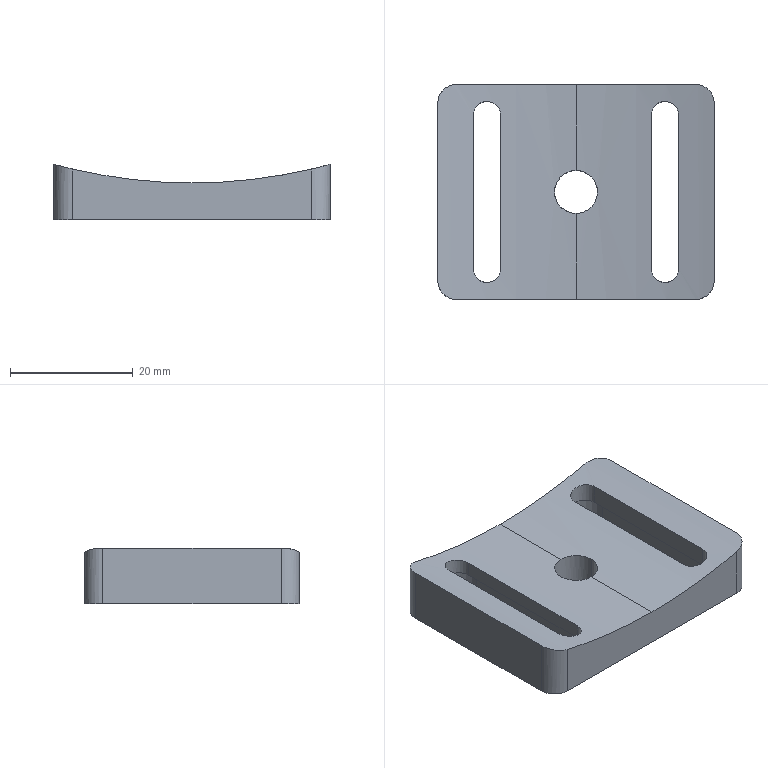Part | SolidWorks | features ICE 2, Extrusion 1, Fillet 1, HoleWzd 1 | 1 solid | 31 faces | box 45 x 35 x 9.032 mm | volume 7770 mm3 | cylinder 16 | plane 15 | commonest cylinder face diameters 4.5 x4 6 x4 8 x4 7 x2 170 x2
STEP:
#1=CARTESIAN_POINT('',(3.5,17.5,-84.928));
#2=VERTEX_POINT('',#1);
#3=CARTESIAN_POINT('',(0.,14.,-85.));
#4=VERTEX_POINT('',#3);
#5=CARTESIAN_POINT('',(3.5,17.5,-84.928));
#6=CARTESIAN_POINT('',(3.5,17.271,-84.928));
#7=CARTESIAN_POINT('',(3.478,17.044,-84.929));
#8=CARTESIAN_POINT('',(3.388,16.593,-84.932));
#9=CARTESIAN_POINT('',(3.321,16.372,-84.935));
#10=CARTESIAN_POINT('',(3.146,15.95,-84.942));
#11=CARTESIAN_POINT('',(3.038,15.747,-84.946));
#12=CARTESIAN_POINT('',(2.782,15.364,-84.955));
#13=CARTESIAN_POINT('',(2.637,15.187,-84.959));
#14=CARTESIAN_POINT('',(2.314,14.864,-84.969));
#15=CARTESIAN_POINT('',(2.134,14.717,-84.973));
#16=CARTESIAN_POINT('',(1.753,14.462,-84.982));
#17=CARTESIAN_POINT('',(1.552,14.355,-84.986));
#18=CARTESIAN_POINT('',(1.129,14.179,-84.993));
#19=CARTESIAN_POINT('',(0.906,14.112,-84.995));
#20=CARTESIAN_POINT('',(0.4583,14.023,-84.999));
#21=CARTESIAN_POINT('',(0.231,14.,-85.));
#22=CARTESIAN_POINT('',(0.,14.,-85.));
#23=B_SPLINE_CURVE_WITH_KNOTS('',3,(#5,#6,#7,#8,#9,#10,#11,#12,#13,#14,#15,#16,#17,#18,#19,#20,#21,#22),.UNSPECIFIED.,.F.,.F.,(4,2,2,2,2,2,2,2,4),(0.01094,0.01163,0.01231,0.013,0.01368,0.01436,0.01505,0.01573,0.01642),.UNSPECIFIED.);
#24=EDGE_CURVE('',#2,#4,#23,.T.);
#25=ORIENTED_EDGE('',*,*,#24,.F.);
#26=CARTESIAN_POINT('',(3.5,17.5,-91.));
#27=VERTEX_POINT('',#26);
#28=CARTESIAN_POINT('',(3.5,17.5,-91.));
#29=DIRECTION('',(0.,0.,-1.));
#30=VECTOR('',#29,1000.);
#31=LINE('',#28,#30);
#32=EDGE_CURVE('',#2,#27,#31,.T.);
#33=ORIENTED_EDGE('',*,*,#32,.T.);
#34=CARTESIAN_POINT('',(-3.5,17.5,-91.));
#35=VERTEX_POINT('',#34);
#36=CARTESIAN_POINT('',(0.,17.5,-91.));
#37=DIRECTION('',(0.,0.,-1.));
#38=DIRECTION('',(-1.,0.,0.));
#39=AXIS2_PLACEMENT_3D('',#36,#37,#38);
#40=CIRCLE('',#39,3.5);
#41=EDGE_CURVE('',#27,#35,#40,.T.);
#42=ORIENTED_EDGE('',*,*,#41,.T.);
#43=CARTESIAN_POINT('',(-3.5,17.5,-84.928));
#44=VERTEX_POINT('',#43);
#45=CARTESIAN_POINT('',(-3.5,17.5,-91.));
#46=DIRECTION('',(0.,0.,-1.));
#47=VECTOR('',#46,1000.);
#48=LINE('',#45,#47);
#49=EDGE_CURVE('',#44,#35,#48,.T.);
#50=ORIENTED_EDGE('',*,*,#49,.F.);
#51=CARTESIAN_POINT('',(0.,14.,-85.));
#52=CARTESIAN_POINT('',(-0.2307,14.,-85.));
#53=CARTESIAN_POINT('',(-0.4588,14.023,-84.999));
#54=CARTESIAN_POINT('',(-0.9058,14.112,-84.995));
#55=CARTESIAN_POINT('',(-1.128,14.179,-84.993));
#56=CARTESIAN_POINT('',(-1.552,14.354,-84.986));
#57=CARTESIAN_POINT('',(-1.753,14.462,-84.982));
#58=CARTESIAN_POINT('',(-2.133,14.715,-84.973));
#59=CARTESIAN_POINT('',(-2.313,14.863,-84.969));
#60=CARTESIAN_POINT('',(-2.636,15.186,-84.959));
#61=CARTESIAN_POINT('',(-2.78,15.362,-84.955));
#62=CARTESIAN_POINT('',(-3.036,15.743,-84.946));
#63=CARTESIAN_POINT('',(-3.145,15.947,-84.942));
#64=CARTESIAN_POINT('',(-3.407,16.579,-84.932));
#65=CARTESIAN_POINT('',(-3.5,17.038,-84.928));
#66=CARTESIAN_POINT('',(-3.5,17.5,-84.928));
#67=B_SPLINE_CURVE_WITH_KNOTS('',3,(#51,#52,#53,#54,#55,#56,#57,#58,#59,#60,#61,#62,#63,#64,#65,#66),.UNSPECIFIED.,.F.,.F.,(4,2,2,2,2,2,2,4),(0.01642,0.0171,0.01778,0.01847,0.01915,0.01983,0.02052,0.02189),.UNSPECIFIED.);
#68=EDGE_CURVE('',#4,#44,#67,.T.);
#69=ORIENTED_EDGE('',*,*,#68,.F.);
#70=EDGE_LOOP('',(#25,#33,#42,#50,#69));
#71=FACE_OUTER_BOUND('',#70,.T.);
#72=CARTESIAN_POINT('',(0.,17.5,-91.));
#73=DIRECTION('',(0.,0.,-1.));
#74=DIRECTION('',(-1.,0.,0.));
#75=AXIS2_PLACEMENT_3D('',#72,#73,#74);
#76=CYLINDRICAL_SURFACE('',#75,3.5);
#77=ADVANCED_FACE('',(#71),#76,.F.);
#78=CARTESIAN_POINT('',(12.25,5.,-84.113));
#79=VERTEX_POINT('',#78);
#80=CARTESIAN_POINT('',(12.25,30.,-84.113));
#81=VERTEX_POINT('',#80);
#82=CARTESIAN_POINT('',(12.25,35.,-84.113));
#83=DIRECTION('',(0.,1.,0.));
#84=VECTOR('',#83,1000.);
#85=LINE('',#82,#84);
#86=EDGE_CURVE('',#79,#81,#85,.T.);
#87=ORIENTED_EDGE('',*,*,#86,.T.);
#88=CARTESIAN_POINT('',(16.75,30.,-83.333));
#89=VERTEX_POINT('',#88);
#90=CARTESIAN_POINT('',(12.25,30.,-84.113));
#91=CARTESIAN_POINT('',(12.25,30.15,-84.113));
#92=CARTESIAN_POINT('',(12.265,30.297,-84.11));
#93=CARTESIAN_POINT('',(12.323,30.587,-84.102));
#94=CARTESIAN_POINT('',(12.367,30.73,-84.096));
#95=CARTESIAN_POINT('',(12.481,31.004,-84.079));
#96=CARTESIAN_POINT('',(12.551,31.134,-84.068));
#97=CARTESIAN_POINT('',(12.716,31.379,-84.044));
#98=CARTESIAN_POINT('',(12.812,31.494,-84.029));
#99=CARTESIAN_POINT('',(13.125,31.805,-83.981));
#100=CARTESIAN_POINT('',(13.376,31.971,-83.941));
#101=CARTESIAN_POINT('',(13.782,32.137,-83.875));
#102=CARTESIAN_POINT('',(13.924,32.18,-83.852));
#103=CARTESIAN_POINT('',(14.212,32.236,-83.804));
#104=CARTESIAN_POINT('',(14.357,32.25,-83.779));
#105=CARTESIAN_POINT('',(14.648,32.25,-83.728));
#106=CARTESIAN_POINT('',(14.796,32.235,-83.702));
#107=CARTESIAN_POINT('',(15.082,32.178,-83.651));
#108=CARTESIAN_POINT('',(15.222,32.136,-83.626));
#109=CARTESIAN_POINT('',(15.492,32.025,-83.576));
#110=CARTESIAN_POINT('',(15.623,31.955,-83.552));
#111=CARTESIAN_POINT('',(15.866,31.794,-83.506));
#112=CARTESIAN_POINT('',(15.98,31.701,-83.484));
#113=CARTESIAN_POINT('',(16.19,31.493,-83.444));
#114=CARTESIAN_POINT('',(16.284,31.379,-83.426));
#115=CARTESIAN_POINT('',(16.448,31.136,-83.393));
#116=CARTESIAN_POINT('',(16.519,31.004,-83.379));
#117=CARTESIAN_POINT('',(16.633,30.73,-83.357));
#118=CARTESIAN_POINT('',(16.676,30.59,-83.348));
#119=CARTESIAN_POINT('',(16.735,30.3,-83.336));
#120=CARTESIAN_POINT('',(16.75,30.15,-83.333));
#121=CARTESIAN_POINT('',(16.75,30.,-83.333));
#122=B_SPLINE_CURVE_WITH_KNOTS('',3,(#90,#91,#92,#93,#94,#95,#96,#97,#98,#99,#100,#101,#102,#103,#104,#105,#106,#107,#108,#109,#110,#111,#112,#113,#114,#115,#116,#117,#118,#119,#120,#121),.UNSPECIFIED.,.F.,.F.,(4,2,2,2,2,2,2,2,2,2,2,2,2,2,2,4),(0.,0.0004429,0.0008859,0.001329,0.001772,0.002658,0.003101,0.003543,0.003986,0.004429,0.004872,0.005315,0.005758,0.006201,0.006644,0.007087),.UNSPECIFIED.);
#123=EDGE_CURVE('',#81,#89,#122,.T.);
#124=ORIENTED_EDGE('',*,*,#123,.T.);
#125=CARTESIAN_POINT('',(16.75,5.,-83.333));
#126=VERTEX_POINT('',#125);
#127=CARTESIAN_POINT('',(16.75,35.,-83.333));
#128=DIRECTION('',(0.,-1.,0.));
#129=VECTOR('',#128,1000.);
#130=LINE('',#127,#129);
#131=EDGE_CURVE('',#89,#126,#130,.T.);
#132=ORIENTED_EDGE('',*,*,#131,.T.);
#133=CARTESIAN_POINT('',(16.75,5.,-83.333));
#134=CARTESIAN_POINT('',(16.75,4.852,-83.333));
#135=CARTESIAN_POINT('',(16.736,4.705,-83.336));
#136=CARTESIAN_POINT('',(16.677,4.413,-83.348));
#137=CARTESIAN_POINT('',(16.633,4.27,-83.357));
#138=CARTESIAN_POINT('',(16.52,3.998,-83.379));
#139=CARTESIAN_POINT('',(16.45,3.867,-83.393));
#140=CARTESIAN_POINT('',(16.284,3.621,-83.426));
#141=CARTESIAN_POINT('',(16.191,3.508,-83.444));
#142=CARTESIAN_POINT('',(15.983,3.301,-83.484));
#143=CARTESIAN_POINT('',(15.867,3.207,-83.506));
#144=CARTESIAN_POINT('',(15.624,3.045,-83.552));
#145=CARTESIAN_POINT('',(15.495,2.977,-83.576));
#146=CARTESIAN_POINT('',(15.224,2.865,-83.626));
#147=CARTESIAN_POINT('',(15.082,2.822,-83.651));
#148=CARTESIAN_POINT('',(14.797,2.765,-83.702));
#149=CARTESIAN_POINT('',(14.652,2.75,-83.728));
#150=CARTESIAN_POINT('',(14.357,2.75,-83.779));
#151=CARTESIAN_POINT('',(14.212,2.764,-83.804));
#152=CARTESIAN_POINT('',(13.926,2.82,-83.852));
#153=CARTESIAN_POINT('',(13.784,2.862,-83.875));
#154=CARTESIAN_POINT('',(13.512,2.973,-83.919));
#155=CARTESIAN_POINT('',(13.383,3.042,-83.94));
#156=CARTESIAN_POINT('',(13.138,3.203,-83.979));
#157=CARTESIAN_POINT('',(13.021,3.298,-83.997));
#158=CARTESIAN_POINT('',(12.812,3.505,-84.029));
#159=CARTESIAN_POINT('',(12.718,3.618,-84.043));
#160=CARTESIAN_POINT('',(12.553,3.863,-84.068));
#161=CARTESIAN_POINT('',(12.481,3.995,-84.079));
#162=CARTESIAN_POINT('',(12.311,4.403,-84.104));
#163=CARTESIAN_POINT('',(12.25,4.7,-84.113));
#164=CARTESIAN_POINT('',(12.25,5.,-84.113));
#165=B_SPLINE_CURVE_WITH_KNOTS('',3,(#133,#134,#135,#136,#137,#138,#139,#140,#141,#142,#143,#144,#145,#146,#147,#148,#149,#150,#151,#152,#153,#154,#155,#156,#157,#158,#159,#160,#161,#162,#163,#164),.UNSPECIFIED.,.F.,.F.,(4,2,2,2,2,2,2,2,2,2,2,2,2,2,2,4),(0.007088,0.007531,0.007974,0.008417,0.00886,0.009303,0.009746,0.01019,0.01063,0.01107,0.01152,0.01196,0.0124,0.01285,0.01329,0.01417),.UNSPECIFIED.);
#166=EDGE_CURVE('',#126,#79,#165,.T.);
#167=ORIENTED_EDGE('',*,*,#166,.T.);
#168=EDGE_LOOP('',(#87,#124,#132,#167));
#169=FACE_BOUND('',#168,.T.);
#170=CARTESIAN_POINT('',(0.,35.,-85.));
#171=VERTEX_POINT('',#170);
#172=CARTESIAN_POINT('',(19.5,35.,-82.733));
#173=VERTEX_POINT('',#172);
#174=CARTESIAN_POINT('',(0.,35.,0.));
#175=DIRECTION('',(0.,-1.,0.));
#176=DIRECTION('',(0.,0.,1.));
#177=AXIS2_PLACEMENT_3D('',#174,#175,#176);
#178=CIRCLE('',#177,85.);
#179=EDGE_CURVE('',#171,#173,#178,.T.);
#180=ORIENTED_EDGE('',*,*,#179,.F.);
#181=CARTESIAN_POINT('',(0.,21.,-85.));
#182=VERTEX_POINT('',#181);
#183=CARTESIAN_POINT('',(0.,35.,-85.));
#184=DIRECTION('',(0.,-1.,0.));
#185=VECTOR('',#184,1000.);
#186=LINE('',#183,#185);
#187=EDGE_CURVE('',#171,#182,#186,.T.);
#188=ORIENTED_EDGE('',*,*,#187,.T.);
#189=CARTESIAN_POINT('',(0.,21.,-85.));
#190=CARTESIAN_POINT('',(0.2283,21.,-85.));
#191=CARTESIAN_POINT('',(0.4601,20.977,-84.999));
#192=CARTESIAN_POINT('',(0.9089,20.888,-84.995));
#193=CARTESIAN_POINT('',(1.127,20.822,-84.993));
#194=CARTESIAN_POINT('',(1.551,20.646,-84.986));
#195=CARTESIAN_POINT('',(1.756,20.536,-84.982));
#196=CARTESIAN_POINT('',(2.135,20.283,-84.973));
#197=CARTESIAN_POINT('',(2.311,20.138,-84.969));
#198=CARTESIAN_POINT('',(2.638,19.812,-84.959));
#199=CARTESIAN_POINT('',(2.783,19.635,-84.955));
#200=CARTESIAN_POINT('',(3.036,19.256,-84.946));
#201=CARTESIAN_POINT('',(3.146,19.051,-84.942));
#202=CARTESIAN_POINT('',(3.322,18.627,-84.935));
#203=CARTESIAN_POINT('',(3.388,18.409,-84.932));
#204=CARTESIAN_POINT('',(3.477,17.96,-84.929));
#205=CARTESIAN_POINT('',(3.5,17.728,-84.928));
#206=CARTESIAN_POINT('',(3.5,17.5,-84.928));
#207=B_SPLINE_CURVE_WITH_KNOTS('',3,(#189,#190,#191,#192,#193,#194,#195,#196,#197,#198,#199,#200,#201,#202,#203,#204,#205,#206),.UNSPECIFIED.,.F.,.F.,(4,2,2,2,2,2,2,2,4),(0.005473,0.006157,0.006841,0.007525,0.008208,0.008892,0.009576,0.01026,0.01094),.UNSPECIFIED.);
#208=EDGE_CURVE('',#182,#2,#207,.T.);
#209=ORIENTED_EDGE('',*,*,#208,.T.);
#210=ORIENTED_EDGE('',*,*,#24,.T.);
#211=CARTESIAN_POINT('',(0.,0.,-85.));
#212=VERTEX_POINT('',#211);
#213=CARTESIAN_POINT('',(0.,35.,-85.));
#214=DIRECTION('',(0.,-1.,0.));
#215=VECTOR('',#214,1000.);
#216=LINE('',#213,#215);
#217=EDGE_CURVE('',#4,#212,#216,.T.);
#218=ORIENTED_EDGE('',*,*,#217,.T.);
#219=CARTESIAN_POINT('',(19.5,0.,-82.733));
#220=VERTEX_POINT('',#219);
#221=CARTESIAN_POINT('',(0.,0.,0.));
#222=DIRECTION('',(0.,-1.,0.));
#223=DIRECTION('',(0.,0.,1.));
#224=AXIS2_PLACEMENT_3D('',#221,#222,#223);
#225=CIRCLE('',#224,85.);
#226=EDGE_CURVE('',#212,#220,#225,.T.);
#227=ORIENTED_EDGE('',*,*,#226,.T.);
#228=CARTESIAN_POINT('',(22.5,3.,-81.968));
#229=VERTEX_POINT('',#228);
#230=CARTESIAN_POINT('',(19.5,0.,-82.733));
#231=CARTESIAN_POINT('',(19.696,0.,-82.687));
#232=CARTESIAN_POINT('',(19.888,0.01899,-82.641));
#233=CARTESIAN_POINT('',(20.267,0.09331,-82.549));
#234=CARTESIAN_POINT('',(20.455,0.1494,-82.502));
#235=CARTESIAN_POINT('',(20.816,0.2968,-82.412));
#236=CARTESIAN_POINT('',(20.987,0.3871,-82.369));
#237=CARTESIAN_POINT('',(21.311,0.6007,-82.285));
#238=CARTESIAN_POINT('',(21.466,0.7256,-82.245));
#239=CARTESIAN_POINT('',(21.745,1.,-82.172));
#240=CARTESIAN_POINT('',(21.87,1.15,-82.138));
#241=CARTESIAN_POINT('',(22.092,1.476,-82.079));
#242=CARTESIAN_POINT('',(22.188,1.653,-82.053));
#243=CARTESIAN_POINT('',(22.418,2.198,-81.991));
#244=CARTESIAN_POINT('',(22.5,2.597,-81.968));
#245=CARTESIAN_POINT('',(22.5,3.,-81.968));
#246=B_SPLINE_CURVE_WITH_KNOTS('',3,(#230,#231,#232,#233,#234,#235,#236,#237,#238,#239,#240,#241,#242,#243,#244,#245),.UNSPECIFIED.,.F.,.F.,(4,2,2,2,2,2,2,4),(0.,0.000595,0.00119,0.001785,0.00238,0.002975,0.00357,0.00476),.UNSPECIFIED.);
#247=EDGE_CURVE('',#220,#229,#246,.T.);
#248=ORIENTED_EDGE('',*,*,#247,.T.);
#249=CARTESIAN_POINT('',(22.5,32.,-81.968));
#250=VERTEX_POINT('',#249);
#251=CARTESIAN_POINT('',(22.5,35.,-81.968));
#252=DIRECTION('',(0.,-1.,0.));
#253=VECTOR('',#252,1000.);
#254=LINE('',#251,#253);
#255=EDGE_CURVE('',#250,#229,#254,.T.);
#256=ORIENTED_EDGE('',*,*,#255,.F.);
#257=CARTESIAN_POINT('',(22.5,32.,-81.968));
#258=CARTESIAN_POINT('',(22.5,32.201,-81.968));
#259=CARTESIAN_POINT('',(22.48,32.399,-81.973));
#260=CARTESIAN_POINT('',(22.402,32.787,-81.995));
#261=CARTESIAN_POINT('',(22.342,32.98,-82.011));
#262=CARTESIAN_POINT('',(22.188,33.346,-82.053));
#263=CARTESIAN_POINT('',(22.095,33.519,-82.078));
#264=CARTESIAN_POINT('',(21.873,33.846,-82.138));
#265=CARTESIAN_POINT('',(21.746,33.999,-82.171));
#266=CARTESIAN_POINT('',(21.329,34.41,-82.281));
#267=CARTESIAN_POINT('',(20.995,34.629,-82.367));
#268=CARTESIAN_POINT('',(20.459,34.849,-82.501));
#269=CARTESIAN_POINT('',(20.271,34.906,-82.548));
#270=CARTESIAN_POINT('',(19.889,34.981,-82.641));
#271=CARTESIAN_POINT('',(19.696,35.,-82.687));
#272=CARTESIAN_POINT('',(19.5,35.,-82.733));
#273=B_SPLINE_CURVE_WITH_KNOTS('',3,(#257,#258,#259,#260,#261,#262,#263,#264,#265,#266,#267,#268,#269,#270,#271,#272),.UNSPECIFIED.,.F.,.F.,(4,2,2,2,2,2,2,4),(0.,0.000595,0.00119,0.001785,0.00238,0.00357,0.004165,0.00476),.UNSPECIFIED.);
#274=EDGE_CURVE('',#250,#173,#273,.T.);
#275=ORIENTED_EDGE('',*,*,#274,.T.);
#276=EDGE_LOOP('',(#180,#188,#209,#210,#218,#227,#248,#256,#275));
#277=FACE_OUTER_BOUND('',#276,.T.);
#278=CARTESIAN_POINT('',(0.,35.,0.));
#279=DIRECTION('',(0.,-1.,0.));
#280=DIRECTION('',(0.,0.,-1.));
#281=AXIS2_PLACEMENT_3D('',#278,#279,#280);
#282=CYLINDRICAL_SURFACE('',#281,85.);
#283=ADVANCED_FACE('',(#169,#277),#282,.F.);
#284=CARTESIAN_POINT('',(-12.25,30.,-86.5));
#285=VERTEX_POINT('',#284);
#286=CARTESIAN_POINT('',(-16.75,30.,-86.5));
#287=VERTEX_POINT('',#286);
#288=CARTESIAN_POINT('',(-14.5,30.,-86.5));
#289=DIRECTION('',(0.,0.,1.));
#290=DIRECTION('',(-1.,0.,0.));
#291=AXIS2_PLACEMENT_3D('',#288,#289,#290);
#292=CIRCLE('',#291,2.25);
#293=EDGE_CURVE('',#285,#287,#292,.T.);
#294=ORIENTED_EDGE('',*,*,#293,.F.);
#295=CARTESIAN_POINT('',(-12.25,30.,-84.113));
#296=VERTEX_POINT('',#295);
#297=CARTESIAN_POINT('',(-12.25,30.,-81.785));
#298=DIRECTION('',(0.,0.,-1.));
#299=VECTOR('',#298,1000.);
#300=LINE('',#297,#299);
#301=EDGE_CURVE('',#296,#285,#300,.T.);
#302=ORIENTED_EDGE('',*,*,#301,.F.);
#303=CARTESIAN_POINT('',(-16.75,30.,-83.333));
#304=VERTEX_POINT('',#303);
#305=CARTESIAN_POINT('',(-16.75,30.,-83.333));
#306=CARTESIAN_POINT('',(-16.75,30.15,-83.333));
#307=CARTESIAN_POINT('',(-16.735,30.297,-83.336));
#308=CARTESIAN_POINT('',(-16.677,30.586,-83.348));
#309=CARTESIAN_POINT('',(-16.633,30.73,-83.357));
#310=CARTESIAN_POINT('',(-16.519,31.003,-83.379));
#311=CARTESIAN_POINT('',(-16.45,31.133,-83.393));
#312=CARTESIAN_POINT('',(-16.285,31.378,-83.425));
#313=CARTESIAN_POINT('',(-16.19,31.493,-83.444));
#314=CARTESIAN_POINT('',(-15.878,31.803,-83.504));
#315=CARTESIAN_POINT('',(-15.628,31.969,-83.551));
#316=CARTESIAN_POINT('',(-15.224,32.135,-83.626));
#317=CARTESIAN_POINT('',(-15.083,32.178,-83.651));
#318=CARTESIAN_POINT('',(-14.795,32.235,-83.703));
#319=CARTESIAN_POINT('',(-14.65,32.25,-83.728));
#320=CARTESIAN_POINT('',(-14.359,32.25,-83.779));
#321=CARTESIAN_POINT('',(-14.211,32.236,-83.804));
#322=CARTESIAN_POINT('',(-13.924,32.18,-83.852));
#323=CARTESIAN_POINT('',(-13.784,32.138,-83.875));
#324=CARTESIAN_POINT('',(-13.513,32.027,-83.919));
#325=CARTESIAN_POINT('',(-13.381,31.957,-83.94));
#326=CARTESIAN_POINT('',(-13.137,31.796,-83.979));
#327=CARTESIAN_POINT('',(-13.023,31.703,-83.997));
#328=CARTESIAN_POINT('',(-12.811,31.494,-84.029));
#329=CARTESIAN_POINT('',(-12.717,31.38,-84.043));
#330=CARTESIAN_POINT('',(-12.553,31.137,-84.068));
#331=CARTESIAN_POINT('',(-12.481,31.005,-84.079));
#332=CARTESIAN_POINT('',(-12.367,30.731,-84.096));
#333=CARTESIAN_POINT('',(-12.324,30.59,-84.102));
#334=CARTESIAN_POINT('',(-12.265,30.3,-84.11));
#335=CARTESIAN_POINT('',(-12.25,30.15,-84.113));
#336=CARTESIAN_POINT('',(-12.25,30.,-84.113));
#337=B_SPLINE_CURVE_WITH_KNOTS('',3,(#305,#306,#307,#308,#309,#310,#311,#312,#313,#314,#315,#316,#317,#318,#319,#320,#321,#322,#323,#324,#325,#326,#327,#328,#329,#330,#331,#332,#333,#334,#335,#336),.UNSPECIFIED.,.F.,.F.,(4,2,2,2,2,2,2,2,2,2,2,2,2,2,2,4),(0.,0.0004429,0.0008858,0.001329,0.001772,0.002658,0.0031,0.003543,0.003986,0.004429,0.004872,0.005315,0.005758,0.006201,0.006644,0.007087),.UNSPECIFIED.);
#338=EDGE_CURVE('',#304,#296,#337,.T.);
#339=ORIENTED_EDGE('',*,*,#338,.F.);
#340=CARTESIAN_POINT('',(-16.75,30.,-81.785));
#341=DIRECTION('',(0.,0.,-1.));
#342=VECTOR('',#341,1000.);
#343=LINE('',#340,#342);
#344=EDGE_CURVE('',#304,#287,#343,.T.);
#345=ORIENTED_EDGE('',*,*,#344,.T.);
#346=EDGE_LOOP('',(#294,#302,#339,#345));
#347=FACE_OUTER_BOUND('',#346,.T.);
#348=CARTESIAN_POINT('',(-14.5,30.,-81.785));
#349=DIRECTION('',(0.,0.,-1.));
#350=DIRECTION('',(-1.,0.,0.));
#351=AXIS2_PLACEMENT_3D('',#348,#349,#350);
#352=CYLINDRICAL_SURFACE('',#351,2.25);
#353=ADVANCED_FACE('',(#347),#352,.F.);
#354=CARTESIAN_POINT('',(-16.75,5.,-86.5));
#355=VERTEX_POINT('',#354);
#356=CARTESIAN_POINT('',(-16.75,30.,-86.5));
#357=DIRECTION('',(0.,-1.,0.));
#358=VECTOR('',#357,1000.);
#359=LINE('',#356,#358);
#360=EDGE_CURVE('',#287,#355,#359,.T.);
#361=ORIENTED_EDGE('',*,*,#360,.F.);
#362=ORIENTED_EDGE('',*,*,#344,.F.);
#363=CARTESIAN_POINT('',(-16.75,5.,-83.333));
#364=VERTEX_POINT('',#363);
#365=CARTESIAN_POINT('',(-16.75,35.,-83.333));
#366=DIRECTION('',(0.,1.,0.));
#367=VECTOR('',#366,1000.);
#368=LINE('',#365,#367);
#369=EDGE_CURVE('',#364,#304,#368,.T.);
#370=ORIENTED_EDGE('',*,*,#369,.F.);
#371=CARTESIAN_POINT('',(-16.75,5.,-81.785));
#372=DIRECTION('',(0.,0.,-1.));
#373=VECTOR('',#372,1000.);
#374=LINE('',#371,#373);
#375=EDGE_CURVE('',#364,#355,#374,.T.);
#376=ORIENTED_EDGE('',*,*,#375,.T.);
#377=EDGE_LOOP('',(#361,#362,#370,#376));
#378=FACE_OUTER_BOUND('',#377,.T.);
#379=CARTESIAN_POINT('',(-16.75,30.,-81.785));
#380=DIRECTION('',(-1.,0.,0.));
#381=DIRECTION('',(0.,0.,1.));
#382=AXIS2_PLACEMENT_3D('',#379,#380,#381);
#383=PLANE('',#382);
#384=ADVANCED_FACE('',(#378),#383,.F.);
#385=CARTESIAN_POINT('',(-12.25,5.,-86.5));
#386=VERTEX_POINT('',#385);
#387=CARTESIAN_POINT('',(-14.5,5.,-86.5));
#388=DIRECTION('',(0.,0.,1.));
#389=DIRECTION('',(-1.,0.,0.));
#390=AXIS2_PLACEMENT_3D('',#387,#388,#389);
#391=CIRCLE('',#390,2.25);
#392=EDGE_CURVE('',#355,#386,#391,.T.);
#393=ORIENTED_EDGE('',*,*,#392,.F.);
#394=ORIENTED_EDGE('',*,*,#375,.F.);
#395=CARTESIAN_POINT('',(-12.25,5.,-84.113));
#396=VERTEX_POINT('',#395);
#397=CARTESIAN_POINT('',(-12.25,5.,-84.113));
#398=CARTESIAN_POINT('',(-12.25,4.852,-84.113));
#399=CARTESIAN_POINT('',(-12.264,4.705,-84.111));
#400=CARTESIAN_POINT('',(-12.323,4.413,-84.102));
#401=CARTESIAN_POINT('',(-12.367,4.27,-84.096));
#402=CARTESIAN_POINT('',(-12.537,3.862,-84.07));
#403=CARTESIAN_POINT('',(-12.706,3.61,-84.045));
#404=CARTESIAN_POINT('',(-13.019,3.3,-83.997));
#405=CARTESIAN_POINT('',(-13.135,3.205,-83.979));
#406=CARTESIAN_POINT('',(-13.38,3.043,-83.94));
#407=CARTESIAN_POINT('',(-13.51,2.974,-83.92));
#408=CARTESIAN_POINT('',(-13.782,2.863,-83.875));
#409=CARTESIAN_POINT('',(-13.924,2.82,-83.852));
#410=CARTESIAN_POINT('',(-14.21,2.764,-83.804));
#411=CARTESIAN_POINT('',(-14.355,2.75,-83.779));
#412=CARTESIAN_POINT('',(-14.65,2.75,-83.728));
#413=CARTESIAN_POINT('',(-14.795,2.765,-83.703));
#414=CARTESIAN_POINT('',(-15.08,2.821,-83.652));
#415=CARTESIAN_POINT('',(-15.222,2.864,-83.626));
#416=CARTESIAN_POINT('',(-15.493,2.976,-83.576));
#417=CARTESIAN_POINT('',(-15.622,3.044,-83.552));
#418=CARTESIAN_POINT('',(-15.865,3.206,-83.506));
#419=CARTESIAN_POINT('',(-15.981,3.3,-83.484));
#420=CARTESIAN_POINT('',(-16.189,3.506,-83.444));
#421=CARTESIAN_POINT('',(-16.283,3.619,-83.426));
#422=CARTESIAN_POINT('',(-16.448,3.864,-83.393));
#423=CARTESIAN_POINT('',(-16.519,3.996,-83.379));
#424=CARTESIAN_POINT('',(-16.689,4.403,-83.346));
#425=CARTESIAN_POINT('',(-16.75,4.7,-83.333));
#426=CARTESIAN_POINT('',(-16.75,5.,-83.333));
#427=B_SPLINE_CURVE_WITH_KNOTS('',3,(#397,#398,#399,#400,#401,#402,#403,#404,#405,#406,#407,#408,#409,#410,#411,#412,#413,#414,#415,#416,#417,#418,#419,#420,#421,#422,#423,#424,#425,#426),.UNSPECIFIED.,.F.,.F.,(4,2,2,2,2,2,2,2,2,2,2,2,2,2,4),(0.007088,0.007531,0.007974,0.00886,0.009303,0.009746,0.01019,0.01063,0.01107,0.01152,0.01196,0.0124,0.01285,0.01329,0.01417),.UNSPECIFIED.);
#428=EDGE_CURVE('',#396,#364,#427,.T.);
#429=ORIENTED_EDGE('',*,*,#428,.F.);
#430=CARTESIAN_POINT('',(-12.25,5.,-81.785));
#431=DIRECTION('',(0.,0.,-1.));
#432=VECTOR('',#431,1000.);
#433=LINE('',#430,#432);
#434=EDGE_CURVE('',#396,#386,#433,.T.);
#435=ORIENTED_EDGE('',*,*,#434,.T.);
#436=EDGE_LOOP('',(#393,#394,#429,#435));
#437=FACE_OUTER_BOUND('',#436,.T.);
#438=CARTESIAN_POINT('',(-14.5,5.,-81.785));
#439=DIRECTION('',(0.,0.,-1.));
#440=DIRECTION('',(-1.,0.,0.));
#441=AXIS2_PLACEMENT_3D('',#438,#439,#440);
#442=CYLINDRICAL_SURFACE('',#441,2.25);
#443=ADVANCED_FACE('',(#437),#442,.F.);
#444=CARTESIAN_POINT('',(-12.25,30.,-86.5));
#445=DIRECTION('',(0.,1.,0.));
#446=VECTOR('',#445,1000.);
#447=LINE('',#444,#446);
#448=EDGE_CURVE('',#386,#285,#447,.T.);
#449=ORIENTED_EDGE('',*,*,#448,.F.);
#450=ORIENTED_EDGE('',*,*,#434,.F.);
#451=CARTESIAN_POINT('',(-12.25,35.,-84.113));
#452=DIRECTION('',(0.,-1.,0.));
#453=VECTOR('',#452,1000.);
#454=LINE('',#451,#453);
#455=EDGE_CURVE('',#296,#396,#454,.T.);
#456=ORIENTED_EDGE('',*,*,#455,.F.);
#457=ORIENTED_EDGE('',*,*,#301,.T.);
#458=EDGE_LOOP('',(#449,#450,#456,#457));
#459=FACE_OUTER_BOUND('',#458,.T.);
#460=CARTESIAN_POINT('',(-12.25,30.,-81.785));
#461=DIRECTION('',(1.,0.,0.));
#462=DIRECTION('',(0.,0.,-1.));
#463=AXIS2_PLACEMENT_3D('',#460,#461,#462);
#464=PLANE('',#463);
#465=ADVANCED_FACE('',(#459),#464,.F.);
#466=CARTESIAN_POINT('',(16.75,30.,-86.5));
#467=VERTEX_POINT('',#466);
#468=CARTESIAN_POINT('',(12.25,30.,-86.5));
#469=VERTEX_POINT('',#468);
#470=CARTESIAN_POINT('',(14.5,30.,-86.5));
#471=DIRECTION('',(0.,0.,1.));
#472=DIRECTION('',(-1.,0.,0.));
#473=AXIS2_PLACEMENT_3D('',#470,#471,#472);
#474=CIRCLE('',#473,2.25);
#475=EDGE_CURVE('',#467,#469,#474,.T.);
#476=ORIENTED_EDGE('',*,*,#475,.F.);
#477=CARTESIAN_POINT('',(16.75,30.,-81.785));
#478=DIRECTION('',(0.,0.,-1.));
#479=VECTOR('',#478,1000.);
#480=LINE('',#477,#479);
#481=EDGE_CURVE('',#89,#467,#480,.T.);
#482=ORIENTED_EDGE('',*,*,#481,.F.);
#483=ORIENTED_EDGE('',*,*,#123,.F.);
#484=CARTESIAN_POINT('',(12.25,30.,-81.785));
#485=DIRECTION('',(0.,0.,-1.));
#486=VECTOR('',#485,1000.);
#487=LINE('',#484,#486);
#488=EDGE_CURVE('',#81,#469,#487,.T.);
#489=ORIENTED_EDGE('',*,*,#488,.T.);
#490=EDGE_LOOP('',(#476,#482,#483,#489));
#491=FACE_OUTER_BOUND('',#490,.T.);
#492=CARTESIAN_POINT('',(14.5,30.,-81.785));
#493=DIRECTION('',(0.,0.,-1.));
#494=DIRECTION('',(-1.,0.,0.));
#495=AXIS2_PLACEMENT_3D('',#492,#493,#494);
#496=CYLINDRICAL_SURFACE('',#495,2.25);
#497=ADVANCED_FACE('',(#491),#496,.F.);
#498=CARTESIAN_POINT('',(12.25,5.,-86.5));
#499=VERTEX_POINT('',#498);
#500=CARTESIAN_POINT('',(12.25,30.,-86.5));
#501=DIRECTION('',(0.,-1.,0.));
#502=VECTOR('',#501,1000.);
#503=LINE('',#500,#502);
#504=EDGE_CURVE('',#469,#499,#503,.T.);
#505=ORIENTED_EDGE('',*,*,#504,.F.);
#506=ORIENTED_EDGE('',*,*,#488,.F.);
#507=ORIENTED_EDGE('',*,*,#86,.F.);
#508=CARTESIAN_POINT('',(12.25,5.,-81.785));
#509=DIRECTION('',(0.,0.,-1.));
#510=VECTOR('',#509,1000.);
#511=LINE('',#508,#510);
#512=EDGE_CURVE('',#79,#499,#511,.T.);
#513=ORIENTED_EDGE('',*,*,#512,.T.);
#514=EDGE_LOOP('',(#505,#506,#507,#513));
#515=FACE_OUTER_BOUND('',#514,.T.);
#516=CARTESIAN_POINT('',(12.25,30.,-81.785));
#517=DIRECTION('',(-1.,0.,0.));
#518=DIRECTION('',(0.,0.,1.));
#519=AXIS2_PLACEMENT_3D('',#516,#517,#518);
#520=PLANE('',#519);
#521=ADVANCED_FACE('',(#515),#520,.F.);
#522=CARTESIAN_POINT('',(16.75,5.,-86.5));
#523=VERTEX_POINT('',#522);
#524=CARTESIAN_POINT('',(14.5,5.,-86.5));
#525=DIRECTION('',(0.,0.,1.));
#526=DIRECTION('',(-1.,0.,0.));
#527=AXIS2_PLACEMENT_3D('',#524,#525,#526);
#528=CIRCLE('',#527,2.25);
#529=EDGE_CURVE('',#499,#523,#528,.T.);
#530=ORIENTED_EDGE('',*,*,#529,.F.);
#531=ORIENTED_EDGE('',*,*,#512,.F.);
#532=ORIENTED_EDGE('',*,*,#166,.F.);
#533=CARTESIAN_POINT('',(16.75,5.,-81.785));
#534=DIRECTION('',(0.,0.,-1.));
#535=VECTOR('',#534,1000.);
#536=LINE('',#533,#535);
#537=EDGE_CURVE('',#126,#523,#536,.T.);
#538=ORIENTED_EDGE('',*,*,#537,.T.);
#539=EDGE_LOOP('',(#530,#531,#532,#538));
#540=FACE_OUTER_BOUND('',#539,.T.);
#541=CARTESIAN_POINT('',(14.5,5.,-81.785));
#542=DIRECTION('',(0.,0.,-1.));
#543=DIRECTION('',(-1.,0.,0.));
#544=AXIS2_PLACEMENT_3D('',#541,#542,#543);
#545=CYLINDRICAL_SURFACE('',#544,2.25);
#546=ADVANCED_FACE('',(#540),#545,.F.);
#547=CARTESIAN_POINT('',(16.75,30.,-86.5));
#548=DIRECTION('',(0.,1.,0.));
#549=VECTOR('',#548,1000.);
#550=LINE('',#547,#549);
#551=EDGE_CURVE('',#523,#467,#550,.T.);
#552=ORIENTED_EDGE('',*,*,#551,.F.);
#553=ORIENTED_EDGE('',*,*,#537,.F.);
#554=ORIENTED_EDGE('',*,*,#131,.F.);
#555=ORIENTED_EDGE('',*,*,#481,.T.);
#556=EDGE_LOOP('',(#552,#553,#554,#555));
#557=FACE_OUTER_BOUND('',#556,.T.);
#558=CARTESIAN_POINT('',(16.75,30.,-81.785));
#559=DIRECTION('',(1.,0.,0.));
#560=DIRECTION('',(0.,0.,-1.));
#561=AXIS2_PLACEMENT_3D('',#558,#559,#560);
#562=PLANE('',#561);
#563=ADVANCED_FACE('',(#557),#562,.F.);
#564=CARTESIAN_POINT('',(-10.5,30.,-91.));
#565=VERTEX_POINT('',#564);
#566=CARTESIAN_POINT('',(-10.5,5.,-91.));
#567=VERTEX_POINT('',#566);
#568=CARTESIAN_POINT('',(-10.5,30.,-91.));
#569=DIRECTION('',(0.,-1.,0.));
#570=VECTOR('',#569,1000.);
#571=LINE('',#568,#570);
#572=EDGE_CURVE('',#565,#567,#571,.T.);
#573=ORIENTED_EDGE('',*,*,#572,.F.);
#574=CARTESIAN_POINT('',(-18.5,30.,-91.));
#575=VERTEX_POINT('',#574);
#576=CARTESIAN_POINT('',(-14.5,30.,-91.));
#577=DIRECTION('',(0.,0.,-1.));
#578=DIRECTION('',(-1.,0.,0.));
#579=AXIS2_PLACEMENT_3D('',#576,#577,#578);
#580=CIRCLE('',#579,4.);
#581=EDGE_CURVE('',#575,#565,#580,.T.);
#582=ORIENTED_EDGE('',*,*,#581,.F.);
#583=CARTESIAN_POINT('',(-18.5,5.,-91.));
#584=VERTEX_POINT('',#583);
#585=CARTESIAN_POINT('',(-18.5,30.,-91.));
#586=DIRECTION('',(0.,1.,0.));
#587=VECTOR('',#586,1000.);
#588=LINE('',#585,#587);
#589=EDGE_CURVE('',#584,#575,#588,.T.);
#590=ORIENTED_EDGE('',*,*,#589,.F.);
#591=CARTESIAN_POINT('',(-14.5,5.,-91.));
#592=DIRECTION('',(0.,0.,-1.));
#593=DIRECTION('',(-1.,0.,0.));
#594=AXIS2_PLACEMENT_3D('',#591,#592,#593);
#595=CIRCLE('',#594,4.);
#596=EDGE_CURVE('',#567,#584,#595,.T.);
#597=ORIENTED_EDGE('',*,*,#596,.F.);
#598=EDGE_LOOP('',(#573,#582,#590,#597));
#599=FACE_BOUND('',#598,.T.);
#600=CARTESIAN_POINT('',(18.5,30.,-91.));
#601=VERTEX_POINT('',#600);
#602=CARTESIAN_POINT('',(18.5,5.,-91.));
#603=VERTEX_POINT('',#602);
#604=CARTESIAN_POINT('',(18.5,30.,-91.));
#605=DIRECTION('',(0.,-1.,0.));
#606=VECTOR('',#605,1000.);
#607=LINE('',#604,#606);
#608=EDGE_CURVE('',#601,#603,#607,.T.);
#609=ORIENTED_EDGE('',*,*,#608,.F.);
#610=CARTESIAN_POINT('',(10.5,30.,-91.));
#611=VERTEX_POINT('',#610);
#612=CARTESIAN_POINT('',(14.5,30.,-91.));
#613=DIRECTION('',(0.,0.,-1.));
#614=DIRECTION('',(-1.,0.,0.));
#615=AXIS2_PLACEMENT_3D('',#612,#613,#614);
#616=CIRCLE('',#615,4.);
#617=EDGE_CURVE('',#611,#601,#616,.T.);
#618=ORIENTED_EDGE('',*,*,#617,.F.);
#619=CARTESIAN_POINT('',(10.5,5.,-91.));
#620=VERTEX_POINT('',#619);
#621=CARTESIAN_POINT('',(10.5,30.,-91.));
#622=DIRECTION('',(0.,1.,0.));
#623=VECTOR('',#622,1000.);
#624=LINE('',#621,#623);
#625=EDGE_CURVE('',#620,#611,#624,.T.);
#626=ORIENTED_EDGE('',*,*,#625,.F.);
#627=CARTESIAN_POINT('',(14.5,5.,-91.));
#628=DIRECTION('',(0.,0.,-1.));
#629=DIRECTION('',(-1.,0.,0.));
#630=AXIS2_PLACEMENT_3D('',#627,#628,#629);
#631=CIRCLE('',#630,4.);
#632=EDGE_CURVE('',#603,#620,#631,.T.);
#633=ORIENTED_EDGE('',*,*,#632,.F.);
#634=EDGE_LOOP('',(#609,#618,#626,#633));
#635=FACE_BOUND('',#634,.T.);
#636=CARTESIAN_POINT('',(0.,17.5,-91.));
#637=DIRECTION('',(0.,0.,-1.));
#638=DIRECTION('',(-1.,0.,0.));
#639=AXIS2_PLACEMENT_3D('',#636,#637,#638);
#640=CIRCLE('',#639,3.5);
#641=EDGE_CURVE('',#35,#27,#640,.T.);
#642=ORIENTED_EDGE('',*,*,#641,.F.);
#643=ORIENTED_EDGE('',*,*,#41,.F.);
#644=EDGE_LOOP('',(#642,#643));
#645=FACE_BOUND('',#644,.T.);
#646=CARTESIAN_POINT('',(19.5,0.,-91.));
#647=VERTEX_POINT('',#646);
#648=CARTESIAN_POINT('',(-19.5,0.,-91.));
#649=VERTEX_POINT('',#648);
#650=CARTESIAN_POINT('',(-22.5,0.,-91.));
#651=DIRECTION('',(-1.,0.,0.));
#652=VECTOR('',#651,1000.);
#653=LINE('',#650,#652);
#654=EDGE_CURVE('',#647,#649,#653,.T.);
#655=ORIENTED_EDGE('',*,*,#654,.T.);
#656=CARTESIAN_POINT('',(-22.5,3.,-91.));
#657=VERTEX_POINT('',#656);
#658=CARTESIAN_POINT('',(-19.5,3.,-91.));
#659=DIRECTION('',(0.,0.,-1.));
#660=DIRECTION('',(1.,0.,0.));
#661=AXIS2_PLACEMENT_3D('',#658,#659,#660);
#662=CIRCLE('',#661,3.);
#663=EDGE_CURVE('',#649,#657,#662,.T.);
#664=ORIENTED_EDGE('',*,*,#663,.T.);
#665=CARTESIAN_POINT('',(-22.5,32.,-91.));
#666=VERTEX_POINT('',#665);
#667=CARTESIAN_POINT('',(-22.5,35.,-91.));
#668=DIRECTION('',(0.,-1.,0.));
#669=VECTOR('',#668,1000.);
#670=LINE('',#667,#669);
#671=EDGE_CURVE('',#666,#657,#670,.T.);
#672=ORIENTED_EDGE('',*,*,#671,.F.);
#673=CARTESIAN_POINT('',(-19.5,35.,-91.));
#674=VERTEX_POINT('',#673);
#675=CARTESIAN_POINT('',(-19.5,32.,-91.));
#676=DIRECTION('',(0.,0.,-1.));
#677=DIRECTION('',(1.,0.,0.));
#678=AXIS2_PLACEMENT_3D('',#675,#676,#677);
#679=CIRCLE('',#678,3.);
#680=EDGE_CURVE('',#666,#674,#679,.T.);
#681=ORIENTED_EDGE('',*,*,#680,.T.);
#682=CARTESIAN_POINT('',(19.5,35.,-91.));
#683=VERTEX_POINT('',#682);
#684=CARTESIAN_POINT('',(-22.5,35.,-91.));
#685=DIRECTION('',(-1.,0.,0.));
#686=VECTOR('',#685,1000.);
#687=LINE('',#684,#686);
#688=EDGE_CURVE('',#683,#674,#687,.T.);
#689=ORIENTED_EDGE('',*,*,#688,.F.);
#690=CARTESIAN_POINT('',(22.5,32.,-91.));
#691=VERTEX_POINT('',#690);
#692=CARTESIAN_POINT('',(19.5,32.,-91.));
#693=DIRECTION('',(0.,0.,-1.));
#694=DIRECTION('',(1.,0.,0.));
#695=AXIS2_PLACEMENT_3D('',#692,#693,#694);
#696=CIRCLE('',#695,3.);
#697=EDGE_CURVE('',#683,#691,#696,.T.);
#698=ORIENTED_EDGE('',*,*,#697,.T.);
#699=CARTESIAN_POINT('',(22.5,3.,-91.));
#700=VERTEX_POINT('',#699);
#701=CARTESIAN_POINT('',(22.5,35.,-91.));
#702=DIRECTION('',(0.,-1.,0.));
#703=VECTOR('',#702,1000.);
#704=LINE('',#701,#703);
#705=EDGE_CURVE('',#691,#700,#704,.T.);
#706=ORIENTED_EDGE('',*,*,#705,.T.);
#707=CARTESIAN_POINT('',(19.5,3.,-91.));
#708=DIRECTION('',(0.,0.,-1.));
#709=DIRECTION('',(1.,0.,0.));
#710=AXIS2_PLACEMENT_3D('',#707,#708,#709);
#711=CIRCLE('',#710,3.);
#712=EDGE_CURVE('',#700,#647,#711,.T.);
#713=ORIENTED_EDGE('',*,*,#712,.T.);
#714=EDGE_LOOP('',(#655,#664,#672,#681,#689,#698,#706,#713));
#715=FACE_OUTER_BOUND('',#714,.T.);
#716=CARTESIAN_POINT('',(-22.5,35.,-91.));
#717=DIRECTION('',(0.,0.,1.));
#718=DIRECTION('',(1.,0.,0.));
#719=AXIS2_PLACEMENT_3D('',#716,#717,#718);
#720=PLANE('',#719);
#721=ADVANCED_FACE('',(#599,#635,#645,#715),#720,.F.);
#722=ORIENTED_EDGE('',*,*,#671,.T.);
#723=CARTESIAN_POINT('',(-22.5,3.,-81.968));
#724=VERTEX_POINT('',#723);
#725=CARTESIAN_POINT('',(-22.5,3.,-81.968));
#726=DIRECTION('',(0.,0.,1.));
#727=VECTOR('',#726,1000.);
#728=LINE('',#725,#727);
#729=EDGE_CURVE('',#657,#724,#728,.T.);
#730=ORIENTED_EDGE('',*,*,#729,.T.);
#731=CARTESIAN_POINT('',(-22.5,32.,-81.968));
#732=VERTEX_POINT('',#731);
#733=CARTESIAN_POINT('',(-22.5,35.,-81.968));
#734=DIRECTION('',(0.,-1.,0.));
#735=VECTOR('',#734,1000.);
#736=LINE('',#733,#735);
#737=EDGE_CURVE('',#732,#724,#736,.T.);
#738=ORIENTED_EDGE('',*,*,#737,.F.);
#739=CARTESIAN_POINT('',(-22.5,32.,-91.));
#740=DIRECTION('',(0.,0.,-1.));
#741=VECTOR('',#740,1000.);
#742=LINE('',#739,#741);
#743=EDGE_CURVE('',#732,#666,#742,.T.);
#744=ORIENTED_EDGE('',*,*,#743,.T.);
#745=EDGE_LOOP('',(#722,#730,#738,#744));
#746=FACE_OUTER_BOUND('',#745,.T.);
#747=CARTESIAN_POINT('',(-22.5,35.,-81.968));
#748=DIRECTION('',(1.,0.,0.));
#749=DIRECTION('',(0.,0.,-1.));
#750=AXIS2_PLACEMENT_3D('',#747,#748,#749);
#751=PLANE('',#750);
#752=ADVANCED_FACE('',(#746),#751,.F.);
#753=ORIENTED_EDGE('',*,*,#187,.F.);
#754=CARTESIAN_POINT('',(-19.5,35.,-82.733));
#755=VERTEX_POINT('',#754);
#756=CARTESIAN_POINT('',(0.,35.,0.));
#757=DIRECTION('',(0.,-1.,0.));
#758=DIRECTION('',(0.,0.,1.));
#759=AXIS2_PLACEMENT_3D('',#756,#757,#758);
#760=CIRCLE('',#759,85.);
#761=EDGE_CURVE('',#755,#171,#760,.T.);
#762=ORIENTED_EDGE('',*,*,#761,.F.);
#763=CARTESIAN_POINT('',(-19.5,35.,-82.733));
#764=CARTESIAN_POINT('',(-19.696,35.,-82.687));
#765=CARTESIAN_POINT('',(-19.888,34.981,-82.641));
#766=CARTESIAN_POINT('',(-20.267,34.907,-82.549));
#767=CARTESIAN_POINT('',(-20.455,34.851,-82.502));
#768=CARTESIAN_POINT('',(-20.816,34.703,-82.412));
#769=CARTESIAN_POINT('',(-20.987,34.613,-82.369));
#770=CARTESIAN_POINT('',(-21.311,34.399,-82.285));
#771=CARTESIAN_POINT('',(-21.466,34.274,-82.245));
#772=CARTESIAN_POINT('',(-21.745,34.,-82.172));
#773=CARTESIAN_POINT('',(-21.87,33.85,-82.138));
#774=CARTESIAN_POINT('',(-22.092,33.524,-82.079));
#775=CARTESIAN_POINT('',(-22.188,33.347,-82.053));
#776=CARTESIAN_POINT('',(-22.418,32.802,-81.991));
#777=CARTESIAN_POINT('',(-22.5,32.403,-81.968));
#778=CARTESIAN_POINT('',(-22.5,32.,-81.968));
#779=B_SPLINE_CURVE_WITH_KNOTS('',3,(#763,#764,#765,#766,#767,#768,#769,#770,#771,#772,#773,#774,#775,#776,#777,#778),.UNSPECIFIED.,.F.,.F.,(4,2,2,2,2,2,2,4),(0.,0.000595,0.00119,0.001785,0.00238,0.002975,0.00357,0.00476),.UNSPECIFIED.);
#780=EDGE_CURVE('',#755,#732,#779,.T.);
#781=ORIENTED_EDGE('',*,*,#780,.T.);
#782=ORIENTED_EDGE('',*,*,#737,.T.);
#783=CARTESIAN_POINT('',(-19.5,0.,-82.733));
#784=VERTEX_POINT('',#783);
#785=CARTESIAN_POINT('',(-22.5,3.,-81.968));
#786=CARTESIAN_POINT('',(-22.5,2.799,-81.968));
#787=CARTESIAN_POINT('',(-22.48,2.601,-81.973));
#788=CARTESIAN_POINT('',(-22.402,2.213,-81.995));
#789=CARTESIAN_POINT('',(-22.342,2.02,-82.011));
#790=CARTESIAN_POINT('',(-22.188,1.654,-82.053));
#791=CARTESIAN_POINT('',(-22.095,1.481,-82.078));
#792=CARTESIAN_POINT('',(-21.873,1.154,-82.138));
#793=CARTESIAN_POINT('',(-21.746,1.001,-82.171));
#794=CARTESIAN_POINT('',(-21.329,0.5902,-82.281));
#795=CARTESIAN_POINT('',(-20.995,0.3707,-82.367));
#796=CARTESIAN_POINT('',(-20.459,0.1508,-82.501));
#797=CARTESIAN_POINT('',(-20.271,0.09418,-82.548));
#798=CARTESIAN_POINT('',(-19.889,0.01897,-82.641));
#799=CARTESIAN_POINT('',(-19.696,0.,-82.687));
#800=CARTESIAN_POINT('',(-19.5,0.,-82.733));
#801=B_SPLINE_CURVE_WITH_KNOTS('',3,(#785,#786,#787,#788,#789,#790,#791,#792,#793,#794,#795,#796,#797,#798,#799,#800),.UNSPECIFIED.,.F.,.F.,(4,2,2,2,2,2,2,4),(0.,0.000595,0.00119,0.001785,0.00238,0.00357,0.004165,0.00476),.UNSPECIFIED.);
#802=EDGE_CURVE('',#724,#784,#801,.T.);
#803=ORIENTED_EDGE('',*,*,#802,.T.);
#804=CARTESIAN_POINT('',(0.,0.,0.));
#805=DIRECTION('',(0.,-1.,0.));
#806=DIRECTION('',(0.,0.,1.));
#807=AXIS2_PLACEMENT_3D('',#804,#805,#806);
#808=CIRCLE('',#807,85.);
#809=EDGE_CURVE('',#784,#212,#808,.T.);
#810=ORIENTED_EDGE('',*,*,#809,.T.);
#811=ORIENTED_EDGE('',*,*,#217,.F.);
#812=ORIENTED_EDGE('',*,*,#68,.T.);
#813=CARTESIAN_POINT('',(-3.5,17.5,-84.928));
#814=CARTESIAN_POINT('',(-3.5,17.731,-84.928));
#815=CARTESIAN_POINT('',(-3.477,17.959,-84.929));
#816=CARTESIAN_POINT('',(-3.388,18.406,-84.932));
#817=CARTESIAN_POINT('',(-3.321,18.629,-84.935));
#818=CARTESIAN_POINT('',(-3.145,19.053,-84.942));
#819=CARTESIAN_POINT('',(-3.038,19.254,-84.946));
#820=CARTESIAN_POINT('',(-2.783,19.634,-84.955));
#821=CARTESIAN_POINT('',(-2.636,19.814,-84.959));
#822=CARTESIAN_POINT('',(-2.312,20.137,-84.969));
#823=CARTESIAN_POINT('',(-2.136,20.282,-84.973));
#824=CARTESIAN_POINT('',(-1.753,20.538,-84.982));
#825=CARTESIAN_POINT('',(-1.55,20.647,-84.986));
#826=CARTESIAN_POINT('',(-1.128,20.821,-84.993));
#827=CARTESIAN_POINT('',(-0.9075,20.888,-84.995));
#828=CARTESIAN_POINT('',(-0.4556,20.978,-84.999));
#829=CARTESIAN_POINT('',(-0.2284,21.,-85.));
#830=CARTESIAN_POINT('',(0.,21.,-85.));
#831=B_SPLINE_CURVE_WITH_KNOTS('',3,(#813,#814,#815,#816,#817,#818,#819,#820,#821,#822,#823,#824,#825,#826,#827,#828,#829,#830),.UNSPECIFIED.,.F.,.F.,(4,2,2,2,2,2,2,2,4),(0.,0.0006841,0.001368,0.002052,0.002737,0.003421,0.004105,0.004789,0.005473),.UNSPECIFIED.);
#832=EDGE_CURVE('',#44,#182,#831,.T.);
#833=ORIENTED_EDGE('',*,*,#832,.T.);
#834=EDGE_LOOP('',(#753,#762,#781,#782,#803,#810,#811,#812,#833));
#835=FACE_OUTER_BOUND('',#834,.T.);
#836=ORIENTED_EDGE('',*,*,#369,.T.);
#837=ORIENTED_EDGE('',*,*,#338,.T.);
#838=ORIENTED_EDGE('',*,*,#455,.T.);
#839=ORIENTED_EDGE('',*,*,#428,.T.);
#840=EDGE_LOOP('',(#836,#837,#838,#839));
#841=FACE_BOUND('',#840,.T.);
#842=CARTESIAN_POINT('',(0.,35.,0.));
#843=DIRECTION('',(0.,-1.,0.));
#844=DIRECTION('',(0.,0.,-1.));
#845=AXIS2_PLACEMENT_3D('',#842,#843,#844);
#846=CYLINDRICAL_SURFACE('',#845,85.);
#847=ADVANCED_FACE('',(#835,#841),#846,.F.);
#848=ORIENTED_EDGE('',*,*,#255,.T.);
#849=CARTESIAN_POINT('',(22.5,3.,-91.));
#850=DIRECTION('',(0.,0.,-1.));
#851=VECTOR('',#850,1000.);
#852=LINE('',#849,#851);
#853=EDGE_CURVE('',#229,#700,#852,.T.);
#854=ORIENTED_EDGE('',*,*,#853,.T.);
#855=ORIENTED_EDGE('',*,*,#705,.F.);
#856=CARTESIAN_POINT('',(22.5,32.,-81.968));
#857=DIRECTION('',(0.,0.,1.));
#858=VECTOR('',#857,1000.);
#859=LINE('',#856,#858);
#860=EDGE_CURVE('',#691,#250,#859,.T.);
#861=ORIENTED_EDGE('',*,*,#860,.T.);
#862=EDGE_LOOP('',(#848,#854,#855,#861));
#863=FACE_OUTER_BOUND('',#862,.T.);
#864=CARTESIAN_POINT('',(22.5,35.,-91.));
#865=DIRECTION('',(-1.,0.,0.));
#866=DIRECTION('',(0.,0.,1.));
#867=AXIS2_PLACEMENT_3D('',#864,#865,#866);
#868=PLANE('',#867);
#869=ADVANCED_FACE('',(#863),#868,.F.);
#870=ORIENTED_EDGE('',*,*,#688,.T.);
#871=CARTESIAN_POINT('',(-19.5,35.,-81.968));
#872=DIRECTION('',(0.,0.,1.));
#873=VECTOR('',#872,1000.);
#874=LINE('',#871,#873);
#875=EDGE_CURVE('',#674,#755,#874,.T.);
#876=ORIENTED_EDGE('',*,*,#875,.T.);
#877=ORIENTED_EDGE('',*,*,#761,.T.);
#878=ORIENTED_EDGE('',*,*,#179,.T.);
#879=CARTESIAN_POINT('',(19.5,35.,-91.));
#880=DIRECTION('',(0.,0.,-1.));
#881=VECTOR('',#880,1000.);
#882=LINE('',#879,#881);
#883=EDGE_CURVE('',#173,#683,#882,.T.);
#884=ORIENTED_EDGE('',*,*,#883,.T.);
#885=EDGE_LOOP('',(#870,#876,#877,#878,#884));
#886=FACE_OUTER_BOUND('',#885,.T.);
#887=CARTESIAN_POINT('',(0.,35.,0.));
#888=DIRECTION('',(0.,1.,0.));
#889=DIRECTION('',(0.,0.,1.));
#890=AXIS2_PLACEMENT_3D('',#887,#888,#889);
#891=PLANE('',#890);
#892=ADVANCED_FACE('',(#886),#891,.T.);
#893=ORIENTED_EDGE('',*,*,#809,.F.);
#894=CARTESIAN_POINT('',(-19.5,0.,0.));
#895=DIRECTION('',(0.,0.,-1.));
#896=VECTOR('',#895,1000.);
#897=LINE('',#894,#896);
#898=EDGE_CURVE('',#784,#649,#897,.T.);
#899=ORIENTED_EDGE('',*,*,#898,.T.);
#900=ORIENTED_EDGE('',*,*,#654,.F.);
#901=CARTESIAN_POINT('',(19.5,0.,0.));
#902=DIRECTION('',(0.,0.,1.));
#903=VECTOR('',#902,1000.);
#904=LINE('',#901,#903);
#905=EDGE_CURVE('',#647,#220,#904,.T.);
#906=ORIENTED_EDGE('',*,*,#905,.T.);
#907=ORIENTED_EDGE('',*,*,#226,.F.);
#908=EDGE_LOOP('',(#893,#899,#900,#906,#907));
#909=FACE_OUTER_BOUND('',#908,.T.);
#910=CARTESIAN_POINT('',(0.,0.,0.));
#911=DIRECTION('',(0.,1.,0.));
#912=DIRECTION('',(0.,0.,1.));
#913=AXIS2_PLACEMENT_3D('',#910,#911,#912);
#914=PLANE('',#913);
#915=ADVANCED_FACE('',(#909),#914,.F.);
#916=ORIENTED_EDGE('',*,*,#663,.F.);
#917=ORIENTED_EDGE('',*,*,#898,.F.);
#918=ORIENTED_EDGE('',*,*,#802,.F.);
#919=ORIENTED_EDGE('',*,*,#729,.F.);
#920=EDGE_LOOP('',(#916,#917,#918,#919));
#921=FACE_OUTER_BOUND('',#920,.T.);
#922=CARTESIAN_POINT('',(-19.5,3.,-81.968));
#923=DIRECTION('',(0.,0.,1.));
#924=DIRECTION('',(1.,0.,0.));
#925=AXIS2_PLACEMENT_3D('',#922,#923,#924);
#926=CYLINDRICAL_SURFACE('',#925,3.);
#927=ADVANCED_FACE('',(#921),#926,.T.);
#928=ORIENTED_EDGE('',*,*,#680,.F.);
#929=ORIENTED_EDGE('',*,*,#743,.F.);
#930=ORIENTED_EDGE('',*,*,#780,.F.);
#931=ORIENTED_EDGE('',*,*,#875,.F.);
#932=EDGE_LOOP('',(#928,#929,#930,#931));
#933=FACE_OUTER_BOUND('',#932,.T.);
#934=CARTESIAN_POINT('',(-19.5,32.,0.));
#935=DIRECTION('',(0.,0.,-1.));
#936=DIRECTION('',(-1.,0.,0.));
#937=AXIS2_PLACEMENT_3D('',#934,#935,#936);
#938=CYLINDRICAL_SURFACE('',#937,3.);
#939=ADVANCED_FACE('',(#933),#938,.T.);
#940=ORIENTED_EDGE('',*,*,#247,.F.);
#941=ORIENTED_EDGE('',*,*,#905,.F.);
#942=ORIENTED_EDGE('',*,*,#712,.F.);
#943=ORIENTED_EDGE('',*,*,#853,.F.);
#944=EDGE_LOOP('',(#940,#941,#942,#943));
#945=FACE_OUTER_BOUND('',#944,.T.);
#946=CARTESIAN_POINT('',(19.5,3.,-91.));
#947=DIRECTION('',(0.,0.,-1.));
#948=DIRECTION('',(-1.,0.,0.));
#949=AXIS2_PLACEMENT_3D('',#946,#947,#948);
#950=CYLINDRICAL_SURFACE('',#949,3.);
#951=ADVANCED_FACE('',(#945),#950,.T.);
#952=ORIENTED_EDGE('',*,*,#274,.F.);
#953=ORIENTED_EDGE('',*,*,#860,.F.);
#954=ORIENTED_EDGE('',*,*,#697,.F.);
#955=ORIENTED_EDGE('',*,*,#883,.F.);
#956=EDGE_LOOP('',(#952,#953,#954,#955));
#957=FACE_OUTER_BOUND('',#956,.T.);
#958=CARTESIAN_POINT('',(19.5,32.,0.));
#959=DIRECTION('',(0.,0.,1.));
#960=DIRECTION('',(1.,0.,0.));
#961=AXIS2_PLACEMENT_3D('',#958,#959,#960);
#962=CYLINDRICAL_SURFACE('',#961,3.);
#963=ADVANCED_FACE('',(#957),#962,.T.);
#964=ORIENTED_EDGE('',*,*,#32,.F.);
#965=ORIENTED_EDGE('',*,*,#208,.F.);
#966=ORIENTED_EDGE('',*,*,#832,.F.);
#967=ORIENTED_EDGE('',*,*,#49,.T.);
#968=ORIENTED_EDGE('',*,*,#641,.T.);
#969=EDGE_LOOP('',(#964,#965,#966,#967,#968));
#970=FACE_OUTER_BOUND('',#969,.T.);
#971=CARTESIAN_POINT('',(0.,17.5,-91.));
#972=DIRECTION('',(0.,0.,-1.));
#973=DIRECTION('',(-1.,0.,0.));
#974=AXIS2_PLACEMENT_3D('',#971,#972,#973);
#975=CYLINDRICAL_SURFACE('',#974,3.5);
#976=ADVANCED_FACE('',(#970),#975,.F.);
#977=CARTESIAN_POINT('',(10.5,30.,-86.5));
#978=VERTEX_POINT('',#977);
#979=CARTESIAN_POINT('',(18.5,30.,-86.5));
#980=VERTEX_POINT('',#979);
#981=CARTESIAN_POINT('',(14.5,30.,-86.5));
#982=DIRECTION('',(0.,0.,-1.));
#983=DIRECTION('',(-1.,0.,0.));
#984=AXIS2_PLACEMENT_3D('',#981,#982,#983);
#985=CIRCLE('',#984,4.);
#986=EDGE_CURVE('',#978,#980,#985,.T.);
#987=ORIENTED_EDGE('',*,*,#986,.T.);
#988=CARTESIAN_POINT('',(18.5,5.,-86.5));
#989=VERTEX_POINT('',#988);
#990=CARTESIAN_POINT('',(18.5,30.,-86.5));
#991=DIRECTION('',(0.,-1.,0.));
#992=VECTOR('',#991,1000.);
#993=LINE('',#990,#992);
#994=EDGE_CURVE('',#980,#989,#993,.T.);
#995=ORIENTED_EDGE('',*,*,#994,.T.);
#996=CARTESIAN_POINT('',(10.5,5.,-86.5));
#997=VERTEX_POINT('',#996);
#998=CARTESIAN_POINT('',(14.5,5.,-86.5));
#999=DIRECTION('',(0.,0.,-1.));
#1000=DIRECTION('',(-1.,0.,0.));
#1001=AXIS2_PLACEMENT_3D('',#998,#999,#1000);
#1002=CIRCLE('',#1001,4.);
#1003=EDGE_CURVE('',#989,#997,#1002,.T.);
#1004=ORIENTED_EDGE('',*,*,#1003,.T.);
#1005=CARTESIAN_POINT('',(10.5,30.,-86.5));
#1006=DIRECTION('',(0.,1.,0.));
#1007=VECTOR('',#1006,1000.);
#1008=LINE('',#1005,#1007);
#1009=EDGE_CURVE('',#997,#978,#1008,.T.);
#1010=ORIENTED_EDGE('',*,*,#1009,.T.);
#1011=EDGE_LOOP('',(#987,#995,#1004,#1010));
#1012=FACE_OUTER_BOUND('',#1011,.T.);
#1013=ORIENTED_EDGE('',*,*,#475,.T.);
#1014=ORIENTED_EDGE('',*,*,#504,.T.);
#1015=ORIENTED_EDGE('',*,*,#529,.T.);
#1016=ORIENTED_EDGE('',*,*,#551,.T.);
#1017=EDGE_LOOP('',(#1013,#1014,#1015,#1016));
#1018=FACE_BOUND('',#1017,.T.);
#1019=CARTESIAN_POINT('',(14.5,30.,-86.5));
#1020=DIRECTION('',(0.,0.,-1.));
#1021=DIRECTION('',(-1.,0.,0.));
#1022=AXIS2_PLACEMENT_3D('',#1019,#1020,#1021);
#1023=PLANE('',#1022);
#1024=ADVANCED_FACE('',(#1012,#1018),#1023,.T.);
#1025=ORIENTED_EDGE('',*,*,#617,.T.);
#1026=CARTESIAN_POINT('',(18.5,30.,-86.5));
#1027=DIRECTION('',(0.,0.,-1.));
#1028=VECTOR('',#1027,1000.);
#1029=LINE('',#1026,#1028);
#1030=EDGE_CURVE('',#980,#601,#1029,.T.);
#1031=ORIENTED_EDGE('',*,*,#1030,.F.);
#1032=ORIENTED_EDGE('',*,*,#986,.F.);
#1033=CARTESIAN_POINT('',(10.5,30.,-86.5));
#1034=DIRECTION('',(0.,0.,-1.));
#1035=VECTOR('',#1034,1000.);
#1036=LINE('',#1033,#1035);
#1037=EDGE_CURVE('',#978,#611,#1036,.T.);
#1038=ORIENTED_EDGE('',*,*,#1037,.T.);
#1039=EDGE_LOOP('',(#1025,#1031,#1032,#1038));
#1040=FACE_OUTER_BOUND('',#1039,.T.);
#1041=CARTESIAN_POINT('',(14.5,30.,-86.5));
#1042=DIRECTION('',(0.,0.,-1.));
#1043=DIRECTION('',(-1.,0.,0.));
#1044=AXIS2_PLACEMENT_3D('',#1041,#1042,#1043);
#1045=CYLINDRICAL_SURFACE('',#1044,4.);
#1046=ADVANCED_FACE('',(#1040),#1045,.F.);
#1047=ORIENTED_EDGE('',*,*,#625,.T.);
#1048=ORIENTED_EDGE('',*,*,#1037,.F.);
#1049=ORIENTED_EDGE('',*,*,#1009,.F.);
#1050=CARTESIAN_POINT('',(10.5,5.,-86.5));
#1051=DIRECTION('',(0.,0.,-1.));
#1052=VECTOR('',#1051,1000.);
#1053=LINE('',#1050,#1052);
#1054=EDGE_CURVE('',#997,#620,#1053,.T.);
#1055=ORIENTED_EDGE('',*,*,#1054,.T.);
#1056=EDGE_LOOP('',(#1047,#1048,#1049,#1055));
#1057=FACE_OUTER_BOUND('',#1056,.T.);
#1058=CARTESIAN_POINT('',(10.5,30.,-86.5));
#1059=DIRECTION('',(-1.,0.,0.));
#1060=DIRECTION('',(0.,-1.,0.));
#1061=AXIS2_PLACEMENT_3D('',#1058,#1059,#1060);
#1062=PLANE('',#1061);
#1063=ADVANCED_FACE('',(#1057),#1062,.F.);
#1064=ORIENTED_EDGE('',*,*,#632,.T.);
#1065=ORIENTED_EDGE('',*,*,#1054,.F.);
#1066=ORIENTED_EDGE('',*,*,#1003,.F.);
#1067=CARTESIAN_POINT('',(18.5,5.,-86.5));
#1068=DIRECTION('',(0.,0.,-1.));
#1069=VECTOR('',#1068,1000.);
#1070=LINE('',#1067,#1069);
#1071=EDGE_CURVE('',#989,#603,#1070,.T.);
#1072=ORIENTED_EDGE('',*,*,#1071,.T.);
#1073=EDGE_LOOP('',(#1064,#1065,#1066,#1072));
#1074=FACE_OUTER_BOUND('',#1073,.T.);
#1075=CARTESIAN_POINT('',(14.5,5.,-86.5));
#1076=DIRECTION('',(0.,0.,-1.));
#1077=DIRECTION('',(-1.,0.,0.));
#1078=AXIS2_PLACEMENT_3D('',#1075,#1076,#1077);
#1079=CYLINDRICAL_SURFACE('',#1078,4.);
#1080=ADVANCED_FACE('',(#1074),#1079,.F.);
#1081=ORIENTED_EDGE('',*,*,#608,.T.);
#1082=ORIENTED_EDGE('',*,*,#1071,.F.);
#1083=ORIENTED_EDGE('',*,*,#994,.F.);
#1084=ORIENTED_EDGE('',*,*,#1030,.T.);
#1085=EDGE_LOOP('',(#1081,#1082,#1083,#1084));
#1086=FACE_OUTER_BOUND('',#1085,.T.);
#1087=CARTESIAN_POINT('',(18.5,30.,-86.5));
#1088=DIRECTION('',(1.,0.,0.));
#1089=DIRECTION('',(0.,1.,0.));
#1090=AXIS2_PLACEMENT_3D('',#1087,#1088,#1089);
#1091=PLANE('',#1090);
#1092=ADVANCED_FACE('',(#1086),#1091,.F.);
#1093=CARTESIAN_POINT('',(-18.5,30.,-86.5));
#1094=VERTEX_POINT('',#1093);
#1095=CARTESIAN_POINT('',(-10.5,30.,-86.5));
#1096=VERTEX_POINT('',#1095);
#1097=CARTESIAN_POINT('',(-14.5,30.,-86.5));
#1098=DIRECTION('',(0.,0.,-1.));
#1099=DIRECTION('',(-1.,0.,0.));
#1100=AXIS2_PLACEMENT_3D('',#1097,#1098,#1099);
#1101=CIRCLE('',#1100,4.);
#1102=EDGE_CURVE('',#1094,#1096,#1101,.T.);
#1103=ORIENTED_EDGE('',*,*,#1102,.T.);
#1104=CARTESIAN_POINT('',(-10.5,5.,-86.5));
#1105=VERTEX_POINT('',#1104);
#1106=CARTESIAN_POINT('',(-10.5,30.,-86.5));
#1107=DIRECTION('',(0.,-1.,0.));
#1108=VECTOR('',#1107,1000.);
#1109=LINE('',#1106,#1108);
#1110=EDGE_CURVE('',#1096,#1105,#1109,.T.);
#1111=ORIENTED_EDGE('',*,*,#1110,.T.);
#1112=CARTESIAN_POINT('',(-18.5,5.,-86.5));
#1113=VERTEX_POINT('',#1112);
#1114=CARTESIAN_POINT('',(-14.5,5.,-86.5));
#1115=DIRECTION('',(0.,0.,-1.));
#1116=DIRECTION('',(-1.,0.,0.));
#1117=AXIS2_PLACEMENT_3D('',#1114,#1115,#1116);
#1118=CIRCLE('',#1117,4.);
#1119=EDGE_CURVE('',#1105,#1113,#1118,.T.);
#1120=ORIENTED_EDGE('',*,*,#1119,.T.);
#1121=CARTESIAN_POINT('',(-18.5,30.,-86.5));
#1122=DIRECTION('',(0.,1.,0.));
#1123=VECTOR('',#1122,1000.);
#1124=LINE('',#1121,#1123);
#1125=EDGE_CURVE('',#1113,#1094,#1124,.T.);
#1126=ORIENTED_EDGE('',*,*,#1125,.T.);
#1127=EDGE_LOOP('',(#1103,#1111,#1120,#1126));
#1128=FACE_OUTER_BOUND('',#1127,.T.);
#1129=ORIENTED_EDGE('',*,*,#293,.T.);
#1130=ORIENTED_EDGE('',*,*,#360,.T.);
#1131=ORIENTED_EDGE('',*,*,#392,.T.);
#1132=ORIENTED_EDGE('',*,*,#448,.T.);
#1133=EDGE_LOOP('',(#1129,#1130,#1131,#1132));
#1134=FACE_BOUND('',#1133,.T.);
#1135=CARTESIAN_POINT('',(-14.5,30.,-86.5));
#1136=DIRECTION('',(0.,0.,-1.));
#1137=DIRECTION('',(-1.,0.,0.));
#1138=AXIS2_PLACEMENT_3D('',#1135,#1136,#1137);
#1139=PLANE('',#1138);
#1140=ADVANCED_FACE('',(#1128,#1134),#1139,.T.);
#1141=ORIENTED_EDGE('',*,*,#581,.T.);
#1142=CARTESIAN_POINT('',(-10.5,30.,-86.5));
#1143=DIRECTION('',(0.,0.,-1.));
#1144=VECTOR('',#1143,1000.);
#1145=LINE('',#1142,#1144);
#1146=EDGE_CURVE('',#1096,#565,#1145,.T.);
#1147=ORIENTED_EDGE('',*,*,#1146,.F.);
#1148=ORIENTED_EDGE('',*,*,#1102,.F.);
#1149=CARTESIAN_POINT('',(-18.5,30.,-86.5));
#1150=DIRECTION('',(0.,0.,-1.));
#1151=VECTOR('',#1150,1000.);
#1152=LINE('',#1149,#1151);
#1153=EDGE_CURVE('',#1094,#575,#1152,.T.);
#1154=ORIENTED_EDGE('',*,*,#1153,.T.);
#1155=EDGE_LOOP('',(#1141,#1147,#1148,#1154));
#1156=FACE_OUTER_BOUND('',#1155,.T.);
#1157=CARTESIAN_POINT('',(-14.5,30.,-86.5));
#1158=DIRECTION('',(0.,0.,-1.));
#1159=DIRECTION('',(-1.,0.,0.));
#1160=AXIS2_PLACEMENT_3D('',#1157,#1158,#1159);
#1161=CYLINDRICAL_SURFACE('',#1160,4.);
#1162=ADVANCED_FACE('',(#1156),#1161,.F.);
#1163=ORIENTED_EDGE('',*,*,#589,.T.);
#1164=ORIENTED_EDGE('',*,*,#1153,.F.);
#1165=ORIENTED_EDGE('',*,*,#1125,.F.);
#1166=CARTESIAN_POINT('',(-18.5,5.,-86.5));
#1167=DIRECTION('',(0.,0.,-1.));
#1168=VECTOR('',#1167,1000.);
#1169=LINE('',#1166,#1168);
#1170=EDGE_CURVE('',#1113,#584,#1169,.T.);
#1171=ORIENTED_EDGE('',*,*,#1170,.T.);
#1172=EDGE_LOOP('',(#1163,#1164,#1165,#1171));
#1173=FACE_OUTER_BOUND('',#1172,.T.);
#1174=CARTESIAN_POINT('',(-18.5,30.,-86.5));
#1175=DIRECTION('',(-1.,0.,0.));
#1176=DIRECTION('',(0.,-1.,0.));
#1177=AXIS2_PLACEMENT_3D('',#1174,#1175,#1176);
#1178=PLANE('',#1177);
#1179=ADVANCED_FACE('',(#1173),#1178,.F.);
#1180=ORIENTED_EDGE('',*,*,#596,.T.);
#1181=ORIENTED_EDGE('',*,*,#1170,.F.);
#1182=ORIENTED_EDGE('',*,*,#1119,.F.);
#1183=CARTESIAN_POINT('',(-10.5,5.,-86.5));
#1184=DIRECTION('',(0.,0.,-1.));
#1185=VECTOR('',#1184,1000.);
#1186=LINE('',#1183,#1185);
#1187=EDGE_CURVE('',#1105,#567,#1186,.T.);
#1188=ORIENTED_EDGE('',*,*,#1187,.T.);
#1189=EDGE_LOOP('',(#1180,#1181,#1182,#1188));
#1190=FACE_OUTER_BOUND('',#1189,.T.);
#1191=CARTESIAN_POINT('',(-14.5,5.,-86.5));
#1192=DIRECTION('',(0.,0.,-1.));
#1193=DIRECTION('',(-1.,0.,0.));
#1194=AXIS2_PLACEMENT_3D('',#1191,#1192,#1193);
#1195=CYLINDRICAL_SURFACE('',#1194,4.);
#1196=ADVANCED_FACE('',(#1190),#1195,.F.);
#1197=ORIENTED_EDGE('',*,*,#572,.T.);
#1198=ORIENTED_EDGE('',*,*,#1187,.F.);
#1199=ORIENTED_EDGE('',*,*,#1110,.F.);
#1200=ORIENTED_EDGE('',*,*,#1146,.T.);
#1201=EDGE_LOOP('',(#1197,#1198,#1199,#1200));
#1202=FACE_OUTER_BOUND('',#1201,.T.);
#1203=CARTESIAN_POINT('',(-10.5,30.,-86.5));
#1204=DIRECTION('',(1.,0.,0.));
#1205=DIRECTION('',(0.,0.,-1.));
#1206=AXIS2_PLACEMENT_3D('',#1203,#1204,#1205);
#1207=PLANE('',#1206);
#1208=ADVANCED_FACE('',(#1202),#1207,.F.);
#1209=CLOSED_SHELL('',(#77,#283,#353,#384,#443,#465,#497,#521,#546,#563,#721,#752,#847,#869,#892,#915,#927,#939,#951,#963,#976,#1024,#1046,#1063,#1080,#1092,#1140,#1162,#1179,#1196,#1208));
#1210=MANIFOLD_SOLID_BREP('',#1209);
#1211=CARTESIAN_POINT('',(0.,0.,0.));
#1212=DIRECTION('',(0.,0.,1.));
#1213=DIRECTION('',(1.,0.,0.));
#1214=AXIS2_PLACEMENT_3D('',#1211,#1212,#1213);
#1215=(LENGTH_UNIT()NAMED_UNIT(*)SI_UNIT(.MILLI.,.METRE.));
#1216=UNCERTAINTY_MEASURE_WITH_UNIT(LENGTH_MEASURE(0.00001),#1215,'','');
#1217=(NAMED_UNIT(*)PLANE_ANGLE_UNIT()SI_UNIT($,.RADIAN.));
#1218=(NAMED_UNIT(*)SI_UNIT($,.STERADIAN.)SOLID_ANGLE_UNIT());
#1219=(GEOMETRIC_REPRESENTATION_CONTEXT(3)GLOBAL_UNCERTAINTY_ASSIGNED_CONTEXT((#1216))GLOBAL_UNIT_ASSIGNED_CONTEXT((#1215,#1217,#1218))REPRESENTATION_CONTEXT('',''));
#1220=ADVANCED_BREP_SHAPE_REPRESENTATION('',(#1210,#1214),#1219);